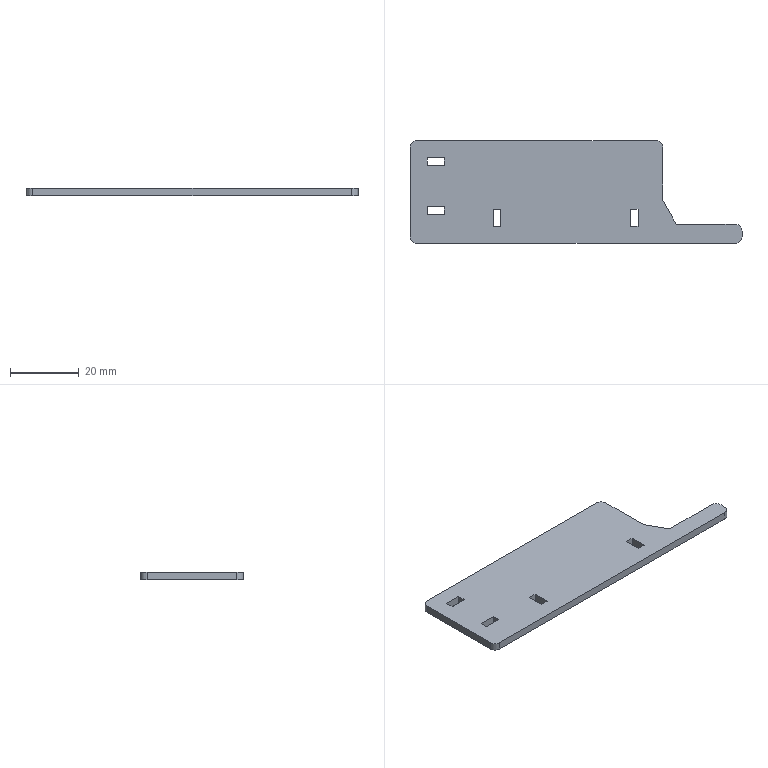Part | SolidWorks | features FlatPattern 1, SMBaseFlange 1, SheetMetal 1 | 1 solid | 31 faces | box 96.8 x 30.001 x 2.3 mm | volume 5301 mm3 | plane 25 | cylinder 6 | commonest cylinder face diameters 4 x6
STEP:
#1=CARTESIAN_POINT('',(1194.712,-717.303,2.3));
#2=VERTEX_POINT('',#1);
#3=CARTESIAN_POINT('',(1196.712,-719.303,2.3));
#4=VERTEX_POINT('',#3);
#5=CARTESIAN_POINT('',(1196.712,-717.303,2.3));
#6=DIRECTION('',(0.,0.,1.));
#7=DIRECTION('',(1.,0.,0.));
#8=AXIS2_PLACEMENT_3D('',#5,#6,#7);
#9=CIRCLE('',#8,2.);
#10=EDGE_CURVE('',#2,#4,#9,.T.);
#11=ORIENTED_EDGE('',*,*,#10,.F.);
#12=CARTESIAN_POINT('',(1194.712,-717.303,0.));
#13=VERTEX_POINT('',#12);
#14=CARTESIAN_POINT('',(1194.712,-717.303,2.3));
#15=DIRECTION('',(0.,0.,-1.));
#16=VECTOR('',#15,1000.);
#17=LINE('',#14,#16);
#18=EDGE_CURVE('',#2,#13,#17,.T.);
#19=ORIENTED_EDGE('',*,*,#18,.T.);
#20=CARTESIAN_POINT('',(1196.712,-719.303,0.));
#21=VERTEX_POINT('',#20);
#22=CARTESIAN_POINT('',(1196.712,-717.303,0.));
#23=DIRECTION('',(0.,0.,1.));
#24=DIRECTION('',(1.,0.,0.));
#25=AXIS2_PLACEMENT_3D('',#22,#23,#24);
#26=CIRCLE('',#25,2.);
#27=EDGE_CURVE('',#13,#21,#26,.T.);
#28=ORIENTED_EDGE('',*,*,#27,.T.);
#29=CARTESIAN_POINT('',(1196.712,-719.303,2.3));
#30=DIRECTION('',(0.,0.,-1.));
#31=VECTOR('',#30,1000.);
#32=LINE('',#29,#31);
#33=EDGE_CURVE('',#4,#21,#32,.T.);
#34=ORIENTED_EDGE('',*,*,#33,.F.);
#35=EDGE_LOOP('',(#11,#19,#28,#34));
#36=FACE_OUTER_BOUND('',#35,.T.);
#37=CARTESIAN_POINT('',(1196.712,-717.303,2.3));
#38=DIRECTION('',(0.,0.,-1.));
#39=DIRECTION('',(-1.,0.,0.));
#40=AXIS2_PLACEMENT_3D('',#37,#38,#39);
#41=CYLINDRICAL_SURFACE('',#40,2.);
#42=ADVANCED_FACE('',(#36),#41,.T.);
#43=CARTESIAN_POINT('',(1272.362,-713.702,2.3));
#44=VERTEX_POINT('',#43);
#45=CARTESIAN_POINT('',(1268.452,-706.712,2.3));
#46=VERTEX_POINT('',#45);
#47=CARTESIAN_POINT('',(1272.362,-713.702,2.3));
#48=DIRECTION('',(-0.4882,0.8727,0.));
#49=VECTOR('',#48,1000.);
#50=LINE('',#47,#49);
#51=EDGE_CURVE('',#44,#46,#50,.T.);
#52=ORIENTED_EDGE('',*,*,#51,.T.);
#53=CARTESIAN_POINT('',(1268.452,-691.303,2.3));
#54=VERTEX_POINT('',#53);
#55=CARTESIAN_POINT('',(1268.452,-706.712,2.3));
#56=DIRECTION('',(0.,1.,0.));
#57=VECTOR('',#56,1000.);
#58=LINE('',#55,#57);
#59=EDGE_CURVE('',#46,#54,#58,.T.);
#60=ORIENTED_EDGE('',*,*,#59,.T.);
#61=CARTESIAN_POINT('',(1266.452,-689.303,2.3));
#62=VERTEX_POINT('',#61);
#63=CARTESIAN_POINT('',(1266.452,-691.303,2.3));
#64=DIRECTION('',(0.,0.,1.));
#65=DIRECTION('',(1.,0.,0.));
#66=AXIS2_PLACEMENT_3D('',#63,#64,#65);
#67=CIRCLE('',#66,2.);
#68=EDGE_CURVE('',#54,#62,#67,.T.);
#69=ORIENTED_EDGE('',*,*,#68,.T.);
#70=CARTESIAN_POINT('',(1196.712,-689.303,2.3));
#71=VERTEX_POINT('',#70);
#72=CARTESIAN_POINT('',(1266.452,-689.303,2.3));
#73=DIRECTION('',(-1.,0.,0.));
#74=VECTOR('',#73,1000.);
#75=LINE('',#72,#74);
#76=EDGE_CURVE('',#62,#71,#75,.T.);
#77=ORIENTED_EDGE('',*,*,#76,.T.);
#78=CARTESIAN_POINT('',(1194.712,-691.303,2.3));
#79=VERTEX_POINT('',#78);
#80=CARTESIAN_POINT('',(1196.712,-691.303,2.3));
#81=DIRECTION('',(0.,0.,1.));
#82=DIRECTION('',(1.,0.,0.));
#83=AXIS2_PLACEMENT_3D('',#80,#81,#82);
#84=CIRCLE('',#83,2.);
#85=EDGE_CURVE('',#71,#79,#84,.T.);
#86=ORIENTED_EDGE('',*,*,#85,.T.);
#87=CARTESIAN_POINT('',(1194.712,-717.303,2.3));
#88=VERTEX_POINT('',#87);
#89=CARTESIAN_POINT('',(1194.712,-691.303,2.3));
#90=DIRECTION('',(-0.00001077,-1.,0.));
#91=VECTOR('',#90,1000.);
#92=LINE('',#89,#91);
#93=EDGE_CURVE('',#79,#88,#92,.T.);
#94=ORIENTED_EDGE('',*,*,#93,.T.);
#95=CARTESIAN_POINT('',(1196.712,-717.303,2.3));
#96=DIRECTION('',(0.,0.,1.));
#97=DIRECTION('',(1.,0.,0.));
#98=AXIS2_PLACEMENT_3D('',#95,#96,#97);
#99=CIRCLE('',#98,2.);
#100=EDGE_CURVE('',#88,#2,#99,.T.);
#101=ORIENTED_EDGE('',*,*,#100,.T.);
#102=ORIENTED_EDGE('',*,*,#10,.T.);
#103=CARTESIAN_POINT('',(1289.512,-719.303,2.3));
#104=VERTEX_POINT('',#103);
#105=CARTESIAN_POINT('',(1196.712,-719.303,2.3));
#106=DIRECTION('',(1.,-0.000005963,0.));
#107=VECTOR('',#106,1000.);
#108=LINE('',#105,#107);
#109=EDGE_CURVE('',#4,#104,#108,.T.);
#110=ORIENTED_EDGE('',*,*,#109,.T.);
#111=CARTESIAN_POINT('',(1291.512,-717.303,2.3));
#112=VERTEX_POINT('',#111);
#113=CARTESIAN_POINT('',(1289.512,-717.303,2.3));
#114=DIRECTION('',(0.,0.,1.));
#115=DIRECTION('',(-1.,0.,0.));
#116=AXIS2_PLACEMENT_3D('',#113,#114,#115);
#117=CIRCLE('',#116,2.);
#118=EDGE_CURVE('',#104,#112,#117,.T.);
#119=ORIENTED_EDGE('',*,*,#118,.T.);
#120=CARTESIAN_POINT('',(1291.512,-715.702,2.3));
#121=VERTEX_POINT('',#120);
#122=CARTESIAN_POINT('',(1291.512,-715.702,2.3));
#123=DIRECTION('',(0.,1.,0.));
#124=VECTOR('',#123,1000.);
#125=LINE('',#122,#124);
#126=EDGE_CURVE('',#112,#121,#125,.T.);
#127=ORIENTED_EDGE('',*,*,#126,.T.);
#128=CARTESIAN_POINT('',(1289.512,-713.702,2.3));
#129=VERTEX_POINT('',#128);
#130=CARTESIAN_POINT('',(1289.512,-715.702,2.3));
#131=DIRECTION('',(0.,0.,1.));
#132=DIRECTION('',(1.,0.,0.));
#133=AXIS2_PLACEMENT_3D('',#130,#131,#132);
#134=CIRCLE('',#133,2.);
#135=EDGE_CURVE('',#121,#129,#134,.T.);
#136=ORIENTED_EDGE('',*,*,#135,.T.);
#137=CARTESIAN_POINT('',(1289.512,-713.702,2.3));
#138=DIRECTION('',(-1.,0.,0.));
#139=VECTOR('',#138,1000.);
#140=LINE('',#137,#139);
#141=EDGE_CURVE('',#129,#44,#140,.T.);
#142=ORIENTED_EDGE('',*,*,#141,.T.);
#143=EDGE_LOOP('',(#52,#60,#69,#77,#86,#94,#101,#102,#110,#119,#127,#136,#142));
#144=FACE_OUTER_BOUND('',#143,.T.);
#145=CARTESIAN_POINT('',(1218.912,-714.303,2.3));
#146=VERTEX_POINT('',#145);
#147=CARTESIAN_POINT('',(1221.212,-714.303,2.3));
#148=VERTEX_POINT('',#147);
#149=CARTESIAN_POINT('',(1218.912,-714.303,2.3));
#150=DIRECTION('',(1.,0.,0.));
#151=VECTOR('',#150,1000.);
#152=LINE('',#149,#151);
#153=EDGE_CURVE('',#146,#148,#152,.T.);
#154=ORIENTED_EDGE('',*,*,#153,.F.);
#155=CARTESIAN_POINT('',(1218.912,-709.303,2.3));
#156=VERTEX_POINT('',#155);
#157=CARTESIAN_POINT('',(1218.912,-709.303,2.3));
#158=DIRECTION('',(0.,-1.,0.));
#159=VECTOR('',#158,1000.);
#160=LINE('',#157,#159);
#161=EDGE_CURVE('',#156,#146,#160,.T.);
#162=ORIENTED_EDGE('',*,*,#161,.F.);
#163=CARTESIAN_POINT('',(1221.212,-709.303,2.3));
#164=VERTEX_POINT('',#163);
#165=CARTESIAN_POINT('',(1218.912,-709.303,2.3));
#166=DIRECTION('',(-1.,0.,0.));
#167=VECTOR('',#166,1000.);
#168=LINE('',#165,#167);
#169=EDGE_CURVE('',#164,#156,#168,.T.);
#170=ORIENTED_EDGE('',*,*,#169,.F.);
#171=CARTESIAN_POINT('',(1221.212,-709.303,2.3));
#172=DIRECTION('',(0.,1.,0.));
#173=VECTOR('',#172,1000.);
#174=LINE('',#171,#173);
#175=EDGE_CURVE('',#148,#164,#174,.T.);
#176=ORIENTED_EDGE('',*,*,#175,.F.);
#177=EDGE_LOOP('',(#154,#162,#170,#176));
#178=FACE_BOUND('',#177,.T.);
#179=CARTESIAN_POINT('',(1258.912,-714.303,2.3));
#180=VERTEX_POINT('',#179);
#181=CARTESIAN_POINT('',(1261.212,-714.303,2.3));
#182=VERTEX_POINT('',#181);
#183=CARTESIAN_POINT('',(1258.912,-714.303,2.3));
#184=DIRECTION('',(1.,0.,0.));
#185=VECTOR('',#184,1000.);
#186=LINE('',#183,#185);
#187=EDGE_CURVE('',#180,#182,#186,.T.);
#188=ORIENTED_EDGE('',*,*,#187,.F.);
#189=CARTESIAN_POINT('',(1258.912,-709.303,2.3));
#190=VERTEX_POINT('',#189);
#191=CARTESIAN_POINT('',(1258.912,-709.303,2.3));
#192=DIRECTION('',(0.,-1.,0.));
#193=VECTOR('',#192,1000.);
#194=LINE('',#191,#193);
#195=EDGE_CURVE('',#190,#180,#194,.T.);
#196=ORIENTED_EDGE('',*,*,#195,.F.);
#197=CARTESIAN_POINT('',(1261.212,-709.303,2.3));
#198=VERTEX_POINT('',#197);
#199=CARTESIAN_POINT('',(1258.912,-709.303,2.3));
#200=DIRECTION('',(-1.,0.,0.));
#201=VECTOR('',#200,1000.);
#202=LINE('',#199,#201);
#203=EDGE_CURVE('',#198,#190,#202,.T.);
#204=ORIENTED_EDGE('',*,*,#203,.F.);
#205=CARTESIAN_POINT('',(1261.212,-709.303,2.3));
#206=DIRECTION('',(0.,1.,0.));
#207=VECTOR('',#206,1000.);
#208=LINE('',#205,#207);
#209=EDGE_CURVE('',#182,#198,#208,.T.);
#210=ORIENTED_EDGE('',*,*,#209,.F.);
#211=EDGE_LOOP('',(#188,#196,#204,#210));
#212=FACE_BOUND('',#211,.T.);
#213=CARTESIAN_POINT('',(1199.712,-696.603,2.3));
#214=VERTEX_POINT('',#213);
#215=CARTESIAN_POINT('',(1204.712,-696.603,2.3));
#216=VERTEX_POINT('',#215);
#217=CARTESIAN_POINT('',(1199.712,-696.603,2.3));
#218=DIRECTION('',(1.,0.,0.));
#219=VECTOR('',#218,1000.);
#220=LINE('',#217,#219);
#221=EDGE_CURVE('',#214,#216,#220,.T.);
#222=ORIENTED_EDGE('',*,*,#221,.F.);
#223=CARTESIAN_POINT('',(1199.712,-694.303,2.3));
#224=VERTEX_POINT('',#223);
#225=CARTESIAN_POINT('',(1199.712,-694.303,2.3));
#226=DIRECTION('',(0.,-1.,0.));
#227=VECTOR('',#226,1000.);
#228=LINE('',#225,#227);
#229=EDGE_CURVE('',#224,#214,#228,.T.);
#230=ORIENTED_EDGE('',*,*,#229,.F.);
#231=CARTESIAN_POINT('',(1204.712,-694.303,2.3));
#232=VERTEX_POINT('',#231);
#233=CARTESIAN_POINT('',(1199.712,-694.303,2.3));
#234=DIRECTION('',(-1.,0.,0.));
#235=VECTOR('',#234,1000.);
#236=LINE('',#233,#235);
#237=EDGE_CURVE('',#232,#224,#236,.T.);
#238=ORIENTED_EDGE('',*,*,#237,.F.);
#239=CARTESIAN_POINT('',(1204.712,-694.303,2.3));
#240=DIRECTION('',(0.,1.,0.));
#241=VECTOR('',#240,1000.);
#242=LINE('',#239,#241);
#243=EDGE_CURVE('',#216,#232,#242,.T.);
#244=ORIENTED_EDGE('',*,*,#243,.F.);
#245=EDGE_LOOP('',(#222,#230,#238,#244));
#246=FACE_BOUND('',#245,.T.);
#247=CARTESIAN_POINT('',(1199.712,-710.903,2.3));
#248=VERTEX_POINT('',#247);
#249=CARTESIAN_POINT('',(1204.712,-710.903,2.3));
#250=VERTEX_POINT('',#249);
#251=CARTESIAN_POINT('',(1199.712,-710.903,2.3));
#252=DIRECTION('',(1.,0.,0.));
#253=VECTOR('',#252,1000.);
#254=LINE('',#251,#253);
#255=EDGE_CURVE('',#248,#250,#254,.T.);
#256=ORIENTED_EDGE('',*,*,#255,.F.);
#257=CARTESIAN_POINT('',(1199.712,-708.603,2.3));
#258=VERTEX_POINT('',#257);
#259=CARTESIAN_POINT('',(1199.712,-708.603,2.3));
#260=DIRECTION('',(0.,-1.,0.));
#261=VECTOR('',#260,1000.);
#262=LINE('',#259,#261);
#263=EDGE_CURVE('',#258,#248,#262,.T.);
#264=ORIENTED_EDGE('',*,*,#263,.F.);
#265=CARTESIAN_POINT('',(1204.712,-708.603,2.3));
#266=VERTEX_POINT('',#265);
#267=CARTESIAN_POINT('',(1199.712,-708.603,2.3));
#268=DIRECTION('',(-1.,0.,0.));
#269=VECTOR('',#268,1000.);
#270=LINE('',#267,#269);
#271=EDGE_CURVE('',#266,#258,#270,.T.);
#272=ORIENTED_EDGE('',*,*,#271,.F.);
#273=CARTESIAN_POINT('',(1204.712,-708.603,2.3));
#274=DIRECTION('',(0.,1.,0.));
#275=VECTOR('',#274,1000.);
#276=LINE('',#273,#275);
#277=EDGE_CURVE('',#250,#266,#276,.T.);
#278=ORIENTED_EDGE('',*,*,#277,.F.);
#279=EDGE_LOOP('',(#256,#264,#272,#278));
#280=FACE_BOUND('',#279,.T.);
#281=CARTESIAN_POINT('',(1266.452,-691.303,2.3));
#282=DIRECTION('',(0.,0.,1.));
#283=DIRECTION('',(1.,0.,0.));
#284=AXIS2_PLACEMENT_3D('',#281,#282,#283);
#285=PLANE('',#284);
#286=ADVANCED_FACE('',(#144,#178,#212,#246,#280),#285,.T.);
#287=CARTESIAN_POINT('',(1199.712,-694.303,0.));
#288=VERTEX_POINT('',#287);
#289=CARTESIAN_POINT('',(1199.712,-696.603,0.));
#290=VERTEX_POINT('',#289);
#291=CARTESIAN_POINT('',(1199.712,-694.303,0.));
#292=DIRECTION('',(0.,-1.,0.));
#293=VECTOR('',#292,1000.);
#294=LINE('',#291,#293);
#295=EDGE_CURVE('',#288,#290,#294,.T.);
#296=ORIENTED_EDGE('',*,*,#295,.T.);
#297=CARTESIAN_POINT('',(1204.712,-696.603,0.));
#298=VERTEX_POINT('',#297);
#299=CARTESIAN_POINT('',(1199.712,-696.603,0.));
#300=DIRECTION('',(1.,0.,0.));
#301=VECTOR('',#300,1000.);
#302=LINE('',#299,#301);
#303=EDGE_CURVE('',#290,#298,#302,.T.);
#304=ORIENTED_EDGE('',*,*,#303,.T.);
#305=CARTESIAN_POINT('',(1204.712,-694.303,0.));
#306=VERTEX_POINT('',#305);
#307=CARTESIAN_POINT('',(1204.712,-694.303,0.));
#308=DIRECTION('',(0.,1.,0.));
#309=VECTOR('',#308,1000.);
#310=LINE('',#307,#309);
#311=EDGE_CURVE('',#298,#306,#310,.T.);
#312=ORIENTED_EDGE('',*,*,#311,.T.);
#313=CARTESIAN_POINT('',(1199.712,-694.303,0.));
#314=DIRECTION('',(-1.,0.,0.));
#315=VECTOR('',#314,1000.);
#316=LINE('',#313,#315);
#317=EDGE_CURVE('',#306,#288,#316,.T.);
#318=ORIENTED_EDGE('',*,*,#317,.T.);
#319=EDGE_LOOP('',(#296,#304,#312,#318));
#320=FACE_BOUND('',#319,.T.);
#321=CARTESIAN_POINT('',(1218.912,-709.303,0.));
#322=VERTEX_POINT('',#321);
#323=CARTESIAN_POINT('',(1218.912,-714.303,0.));
#324=VERTEX_POINT('',#323);
#325=CARTESIAN_POINT('',(1218.912,-709.303,0.));
#326=DIRECTION('',(0.,-1.,0.));
#327=VECTOR('',#326,1000.);
#328=LINE('',#325,#327);
#329=EDGE_CURVE('',#322,#324,#328,.T.);
#330=ORIENTED_EDGE('',*,*,#329,.T.);
#331=CARTESIAN_POINT('',(1221.212,-714.303,0.));
#332=VERTEX_POINT('',#331);
#333=CARTESIAN_POINT('',(1218.912,-714.303,0.));
#334=DIRECTION('',(1.,0.,0.));
#335=VECTOR('',#334,1000.);
#336=LINE('',#333,#335);
#337=EDGE_CURVE('',#324,#332,#336,.T.);
#338=ORIENTED_EDGE('',*,*,#337,.T.);
#339=CARTESIAN_POINT('',(1221.212,-709.303,0.));
#340=VERTEX_POINT('',#339);
#341=CARTESIAN_POINT('',(1221.212,-709.303,0.));
#342=DIRECTION('',(0.,1.,0.));
#343=VECTOR('',#342,1000.);
#344=LINE('',#341,#343);
#345=EDGE_CURVE('',#332,#340,#344,.T.);
#346=ORIENTED_EDGE('',*,*,#345,.T.);
#347=CARTESIAN_POINT('',(1218.912,-709.303,0.));
#348=DIRECTION('',(-1.,0.,0.));
#349=VECTOR('',#348,1000.);
#350=LINE('',#347,#349);
#351=EDGE_CURVE('',#340,#322,#350,.T.);
#352=ORIENTED_EDGE('',*,*,#351,.T.);
#353=EDGE_LOOP('',(#330,#338,#346,#352));
#354=FACE_BOUND('',#353,.T.);
#355=CARTESIAN_POINT('',(1272.362,-713.702,0.));
#356=VERTEX_POINT('',#355);
#357=CARTESIAN_POINT('',(1268.452,-706.712,0.));
#358=VERTEX_POINT('',#357);
#359=CARTESIAN_POINT('',(1272.362,-713.702,0.));
#360=DIRECTION('',(-0.4882,0.8727,0.));
#361=VECTOR('',#360,1000.);
#362=LINE('',#359,#361);
#363=EDGE_CURVE('',#356,#358,#362,.T.);
#364=ORIENTED_EDGE('',*,*,#363,.F.);
#365=CARTESIAN_POINT('',(1289.512,-713.702,0.));
#366=VERTEX_POINT('',#365);
#367=CARTESIAN_POINT('',(1289.512,-713.702,0.));
#368=DIRECTION('',(-1.,0.,0.));
#369=VECTOR('',#368,1000.);
#370=LINE('',#367,#369);
#371=EDGE_CURVE('',#366,#356,#370,.T.);
#372=ORIENTED_EDGE('',*,*,#371,.F.);
#373=CARTESIAN_POINT('',(1291.512,-715.702,0.));
#374=VERTEX_POINT('',#373);
#375=CARTESIAN_POINT('',(1289.512,-715.702,0.));
#376=DIRECTION('',(0.,0.,1.));
#377=DIRECTION('',(1.,0.,0.));
#378=AXIS2_PLACEMENT_3D('',#375,#376,#377);
#379=CIRCLE('',#378,2.);
#380=EDGE_CURVE('',#374,#366,#379,.T.);
#381=ORIENTED_EDGE('',*,*,#380,.F.);
#382=CARTESIAN_POINT('',(1291.512,-717.303,0.));
#383=VERTEX_POINT('',#382);
#384=CARTESIAN_POINT('',(1291.512,-715.702,0.));
#385=DIRECTION('',(0.,1.,0.));
#386=VECTOR('',#385,1000.);
#387=LINE('',#384,#386);
#388=EDGE_CURVE('',#383,#374,#387,.T.);
#389=ORIENTED_EDGE('',*,*,#388,.F.);
#390=CARTESIAN_POINT('',(1289.512,-719.303,0.));
#391=VERTEX_POINT('',#390);
#392=CARTESIAN_POINT('',(1289.512,-717.303,0.));
#393=DIRECTION('',(0.,0.,1.));
#394=DIRECTION('',(-1.,0.,0.));
#395=AXIS2_PLACEMENT_3D('',#392,#393,#394);
#396=CIRCLE('',#395,2.);
#397=EDGE_CURVE('',#391,#383,#396,.T.);
#398=ORIENTED_EDGE('',*,*,#397,.F.);
#399=CARTESIAN_POINT('',(1196.712,-719.303,0.));
#400=DIRECTION('',(1.,-0.000005963,0.));
#401=VECTOR('',#400,1000.);
#402=LINE('',#399,#401);
#403=EDGE_CURVE('',#21,#391,#402,.T.);
#404=ORIENTED_EDGE('',*,*,#403,.F.);
#405=ORIENTED_EDGE('',*,*,#27,.F.);
#406=CARTESIAN_POINT('',(1194.712,-717.303,0.));
#407=VERTEX_POINT('',#406);
#408=CARTESIAN_POINT('',(1196.712,-717.303,0.));
#409=DIRECTION('',(0.,0.,1.));
#410=DIRECTION('',(1.,0.,0.));
#411=AXIS2_PLACEMENT_3D('',#408,#409,#410);
#412=CIRCLE('',#411,2.);
#413=EDGE_CURVE('',#407,#13,#412,.T.);
#414=ORIENTED_EDGE('',*,*,#413,.F.);
#415=CARTESIAN_POINT('',(1194.712,-691.303,0.));
#416=VERTEX_POINT('',#415);
#417=CARTESIAN_POINT('',(1194.712,-691.303,0.));
#418=DIRECTION('',(-0.00001077,-1.,0.));
#419=VECTOR('',#418,1000.);
#420=LINE('',#417,#419);
#421=EDGE_CURVE('',#416,#407,#420,.T.);
#422=ORIENTED_EDGE('',*,*,#421,.F.);
#423=CARTESIAN_POINT('',(1196.712,-689.303,0.));
#424=VERTEX_POINT('',#423);
#425=CARTESIAN_POINT('',(1196.712,-691.303,0.));
#426=DIRECTION('',(0.,0.,1.));
#427=DIRECTION('',(1.,0.,0.));
#428=AXIS2_PLACEMENT_3D('',#425,#426,#427);
#429=CIRCLE('',#428,2.);
#430=EDGE_CURVE('',#424,#416,#429,.T.);
#431=ORIENTED_EDGE('',*,*,#430,.F.);
#432=CARTESIAN_POINT('',(1266.452,-689.303,0.));
#433=VERTEX_POINT('',#432);
#434=CARTESIAN_POINT('',(1266.452,-689.303,0.));
#435=DIRECTION('',(-1.,0.,0.));
#436=VECTOR('',#435,1000.);
#437=LINE('',#434,#436);
#438=EDGE_CURVE('',#433,#424,#437,.T.);
#439=ORIENTED_EDGE('',*,*,#438,.F.);
#440=CARTESIAN_POINT('',(1268.452,-691.303,0.));
#441=VERTEX_POINT('',#440);
#442=CARTESIAN_POINT('',(1266.452,-691.303,0.));
#443=DIRECTION('',(0.,0.,1.));
#444=DIRECTION('',(1.,0.,0.));
#445=AXIS2_PLACEMENT_3D('',#442,#443,#444);
#446=CIRCLE('',#445,2.);
#447=EDGE_CURVE('',#441,#433,#446,.T.);
#448=ORIENTED_EDGE('',*,*,#447,.F.);
#449=CARTESIAN_POINT('',(1268.452,-706.712,0.));
#450=DIRECTION('',(0.,1.,0.));
#451=VECTOR('',#450,1000.);
#452=LINE('',#449,#451);
#453=EDGE_CURVE('',#358,#441,#452,.T.);
#454=ORIENTED_EDGE('',*,*,#453,.F.);
#455=EDGE_LOOP('',(#364,#372,#381,#389,#398,#404,#405,#414,#422,#431,#439,#448,#454));
#456=FACE_OUTER_BOUND('',#455,.T.);
#457=CARTESIAN_POINT('',(1258.912,-709.303,0.));
#458=VERTEX_POINT('',#457);
#459=CARTESIAN_POINT('',(1258.912,-714.303,0.));
#460=VERTEX_POINT('',#459);
#461=CARTESIAN_POINT('',(1258.912,-709.303,0.));
#462=DIRECTION('',(0.,-1.,0.));
#463=VECTOR('',#462,1000.);
#464=LINE('',#461,#463);
#465=EDGE_CURVE('',#458,#460,#464,.T.);
#466=ORIENTED_EDGE('',*,*,#465,.T.);
#467=CARTESIAN_POINT('',(1261.212,-714.303,0.));
#468=VERTEX_POINT('',#467);
#469=CARTESIAN_POINT('',(1258.912,-714.303,0.));
#470=DIRECTION('',(1.,0.,0.));
#471=VECTOR('',#470,1000.);
#472=LINE('',#469,#471);
#473=EDGE_CURVE('',#460,#468,#472,.T.);
#474=ORIENTED_EDGE('',*,*,#473,.T.);
#475=CARTESIAN_POINT('',(1261.212,-709.303,0.));
#476=VERTEX_POINT('',#475);
#477=CARTESIAN_POINT('',(1261.212,-709.303,0.));
#478=DIRECTION('',(0.,1.,0.));
#479=VECTOR('',#478,1000.);
#480=LINE('',#477,#479);
#481=EDGE_CURVE('',#468,#476,#480,.T.);
#482=ORIENTED_EDGE('',*,*,#481,.T.);
#483=CARTESIAN_POINT('',(1258.912,-709.303,0.));
#484=DIRECTION('',(-1.,0.,0.));
#485=VECTOR('',#484,1000.);
#486=LINE('',#483,#485);
#487=EDGE_CURVE('',#476,#458,#486,.T.);
#488=ORIENTED_EDGE('',*,*,#487,.T.);
#489=EDGE_LOOP('',(#466,#474,#482,#488));
#490=FACE_BOUND('',#489,.T.);
#491=CARTESIAN_POINT('',(1199.712,-708.603,0.));
#492=VERTEX_POINT('',#491);
#493=CARTESIAN_POINT('',(1199.712,-710.903,0.));
#494=VERTEX_POINT('',#493);
#495=CARTESIAN_POINT('',(1199.712,-708.603,0.));
#496=DIRECTION('',(0.,-1.,0.));
#497=VECTOR('',#496,1000.);
#498=LINE('',#495,#497);
#499=EDGE_CURVE('',#492,#494,#498,.T.);
#500=ORIENTED_EDGE('',*,*,#499,.T.);
#501=CARTESIAN_POINT('',(1204.712,-710.903,0.));
#502=VERTEX_POINT('',#501);
#503=CARTESIAN_POINT('',(1199.712,-710.903,0.));
#504=DIRECTION('',(1.,0.,0.));
#505=VECTOR('',#504,1000.);
#506=LINE('',#503,#505);
#507=EDGE_CURVE('',#494,#502,#506,.T.);
#508=ORIENTED_EDGE('',*,*,#507,.T.);
#509=CARTESIAN_POINT('',(1204.712,-708.603,0.));
#510=VERTEX_POINT('',#509);
#511=CARTESIAN_POINT('',(1204.712,-708.603,0.));
#512=DIRECTION('',(0.,1.,0.));
#513=VECTOR('',#512,1000.);
#514=LINE('',#511,#513);
#515=EDGE_CURVE('',#502,#510,#514,.T.);
#516=ORIENTED_EDGE('',*,*,#515,.T.);
#517=CARTESIAN_POINT('',(1199.712,-708.603,0.));
#518=DIRECTION('',(-1.,0.,0.));
#519=VECTOR('',#518,1000.);
#520=LINE('',#517,#519);
#521=EDGE_CURVE('',#510,#492,#520,.T.);
#522=ORIENTED_EDGE('',*,*,#521,.T.);
#523=EDGE_LOOP('',(#500,#508,#516,#522));
#524=FACE_BOUND('',#523,.T.);
#525=CARTESIAN_POINT('',(1266.452,-691.303,0.));
#526=DIRECTION('',(0.,0.,1.));
#527=DIRECTION('',(1.,0.,0.));
#528=AXIS2_PLACEMENT_3D('',#525,#526,#527);
#529=PLANE('',#528);
#530=ADVANCED_FACE('',(#320,#354,#456,#490,#524),#529,.F.);
#531=ORIENTED_EDGE('',*,*,#363,.T.);
#532=CARTESIAN_POINT('',(1268.452,-706.712,2.3));
#533=DIRECTION('',(0.,0.,-1.));
#534=VECTOR('',#533,1000.);
#535=LINE('',#532,#534);
#536=EDGE_CURVE('',#46,#358,#535,.T.);
#537=ORIENTED_EDGE('',*,*,#536,.F.);
#538=ORIENTED_EDGE('',*,*,#51,.F.);
#539=CARTESIAN_POINT('',(1272.362,-713.702,2.3));
#540=DIRECTION('',(0.,0.,-1.));
#541=VECTOR('',#540,1000.);
#542=LINE('',#539,#541);
#543=EDGE_CURVE('',#44,#356,#542,.T.);
#544=ORIENTED_EDGE('',*,*,#543,.T.);
#545=EDGE_LOOP('',(#531,#537,#538,#544));
#546=FACE_OUTER_BOUND('',#545,.T.);
#547=CARTESIAN_POINT('',(1272.362,-713.702,2.3));
#548=DIRECTION('',(-0.8727,-0.4882,0.));
#549=DIRECTION('',(0.4882,-0.8727,0.));
#550=AXIS2_PLACEMENT_3D('',#547,#548,#549);
#551=PLANE('',#550);
#552=ADVANCED_FACE('',(#546),#551,.F.);
#553=ORIENTED_EDGE('',*,*,#453,.T.);
#554=CARTESIAN_POINT('',(1268.452,-691.303,2.3));
#555=DIRECTION('',(0.,0.,-1.));
#556=VECTOR('',#555,1000.);
#557=LINE('',#554,#556);
#558=EDGE_CURVE('',#54,#441,#557,.T.);
#559=ORIENTED_EDGE('',*,*,#558,.F.);
#560=ORIENTED_EDGE('',*,*,#59,.F.);
#561=ORIENTED_EDGE('',*,*,#536,.T.);
#562=EDGE_LOOP('',(#553,#559,#560,#561));
#563=FACE_OUTER_BOUND('',#562,.T.);
#564=CARTESIAN_POINT('',(1268.452,-706.712,2.3));
#565=DIRECTION('',(-1.,0.,0.));
#566=DIRECTION('',(0.,-1.,0.));
#567=AXIS2_PLACEMENT_3D('',#564,#565,#566);
#568=PLANE('',#567);
#569=ADVANCED_FACE('',(#563),#568,.F.);
#570=ORIENTED_EDGE('',*,*,#447,.T.);
#571=CARTESIAN_POINT('',(1266.452,-689.303,2.3));
#572=DIRECTION('',(0.,0.,-1.));
#573=VECTOR('',#572,1000.);
#574=LINE('',#571,#573);
#575=EDGE_CURVE('',#62,#433,#574,.T.);
#576=ORIENTED_EDGE('',*,*,#575,.F.);
#577=ORIENTED_EDGE('',*,*,#68,.F.);
#578=ORIENTED_EDGE('',*,*,#558,.T.);
#579=EDGE_LOOP('',(#570,#576,#577,#578));
#580=FACE_OUTER_BOUND('',#579,.T.);
#581=CARTESIAN_POINT('',(1266.452,-691.303,2.3));
#582=DIRECTION('',(0.,0.,-1.));
#583=DIRECTION('',(-1.,0.,0.));
#584=AXIS2_PLACEMENT_3D('',#581,#582,#583);
#585=CYLINDRICAL_SURFACE('',#584,2.);
#586=ADVANCED_FACE('',(#580),#585,.T.);
#587=ORIENTED_EDGE('',*,*,#438,.T.);
#588=CARTESIAN_POINT('',(1196.712,-689.303,2.3));
#589=DIRECTION('',(0.,0.,-1.));
#590=VECTOR('',#589,1000.);
#591=LINE('',#588,#590);
#592=EDGE_CURVE('',#71,#424,#591,.T.);
#593=ORIENTED_EDGE('',*,*,#592,.F.);
#594=ORIENTED_EDGE('',*,*,#76,.F.);
#595=ORIENTED_EDGE('',*,*,#575,.T.);
#596=EDGE_LOOP('',(#587,#593,#594,#595));
#597=FACE_OUTER_BOUND('',#596,.T.);
#598=CARTESIAN_POINT('',(1266.452,-689.303,2.3));
#599=DIRECTION('',(0.,-1.,0.));
#600=DIRECTION('',(1.,0.,0.));
#601=AXIS2_PLACEMENT_3D('',#598,#599,#600);
#602=PLANE('',#601);
#603=ADVANCED_FACE('',(#597),#602,.F.);
#604=ORIENTED_EDGE('',*,*,#430,.T.);
#605=CARTESIAN_POINT('',(1194.712,-691.303,2.3));
#606=DIRECTION('',(0.,0.,-1.));
#607=VECTOR('',#606,1000.);
#608=LINE('',#605,#607);
#609=EDGE_CURVE('',#79,#416,#608,.T.);
#610=ORIENTED_EDGE('',*,*,#609,.F.);
#611=ORIENTED_EDGE('',*,*,#85,.F.);
#612=ORIENTED_EDGE('',*,*,#592,.T.);
#613=EDGE_LOOP('',(#604,#610,#611,#612));
#614=FACE_OUTER_BOUND('',#613,.T.);
#615=CARTESIAN_POINT('',(1196.712,-691.303,2.3));
#616=DIRECTION('',(0.,0.,-1.));
#617=DIRECTION('',(-1.,0.,0.));
#618=AXIS2_PLACEMENT_3D('',#615,#616,#617);
#619=CYLINDRICAL_SURFACE('',#618,2.);
#620=ADVANCED_FACE('',(#614),#619,.T.);
#621=ORIENTED_EDGE('',*,*,#421,.T.);
#622=CARTESIAN_POINT('',(1194.712,-717.303,2.3));
#623=DIRECTION('',(0.,0.,-1.));
#624=VECTOR('',#623,1000.);
#625=LINE('',#622,#624);
#626=EDGE_CURVE('',#88,#407,#625,.T.);
#627=ORIENTED_EDGE('',*,*,#626,.F.);
#628=ORIENTED_EDGE('',*,*,#93,.F.);
#629=ORIENTED_EDGE('',*,*,#609,.T.);
#630=EDGE_LOOP('',(#621,#627,#628,#629));
#631=FACE_OUTER_BOUND('',#630,.T.);
#632=CARTESIAN_POINT('',(1194.712,-691.303,2.3));
#633=DIRECTION('',(1.,-0.00001077,0.));
#634=DIRECTION('',(0.00001077,1.,0.));
#635=AXIS2_PLACEMENT_3D('',#632,#633,#634);
#636=PLANE('',#635);
#637=ADVANCED_FACE('',(#631),#636,.F.);
#638=ORIENTED_EDGE('',*,*,#18,.F.);
#639=ORIENTED_EDGE('',*,*,#100,.F.);
#640=ORIENTED_EDGE('',*,*,#626,.T.);
#641=ORIENTED_EDGE('',*,*,#413,.T.);
#642=EDGE_LOOP('',(#638,#639,#640,#641));
#643=FACE_OUTER_BOUND('',#642,.T.);
#644=CARTESIAN_POINT('',(1196.712,-717.303,2.3));
#645=DIRECTION('',(0.,0.,-1.));
#646=DIRECTION('',(-1.,0.,0.));
#647=AXIS2_PLACEMENT_3D('',#644,#645,#646);
#648=CYLINDRICAL_SURFACE('',#647,2.);
#649=ADVANCED_FACE('',(#643),#648,.T.);
#650=ORIENTED_EDGE('',*,*,#403,.T.);
#651=CARTESIAN_POINT('',(1289.512,-719.303,2.3));
#652=DIRECTION('',(0.,0.,-1.));
#653=VECTOR('',#652,1000.);
#654=LINE('',#651,#653);
#655=EDGE_CURVE('',#104,#391,#654,.T.);
#656=ORIENTED_EDGE('',*,*,#655,.F.);
#657=ORIENTED_EDGE('',*,*,#109,.F.);
#658=ORIENTED_EDGE('',*,*,#33,.T.);
#659=EDGE_LOOP('',(#650,#656,#657,#658));
#660=FACE_OUTER_BOUND('',#659,.T.);
#661=CARTESIAN_POINT('',(1196.712,-719.303,2.3));
#662=DIRECTION('',(0.000005963,1.,0.));
#663=DIRECTION('',(-1.,0.000005963,0.));
#664=AXIS2_PLACEMENT_3D('',#661,#662,#663);
#665=PLANE('',#664);
#666=ADVANCED_FACE('',(#660),#665,.F.);
#667=ORIENTED_EDGE('',*,*,#397,.T.);
#668=CARTESIAN_POINT('',(1291.512,-717.303,2.3));
#669=DIRECTION('',(0.,0.,-1.));
#670=VECTOR('',#669,1000.);
#671=LINE('',#668,#670);
#672=EDGE_CURVE('',#112,#383,#671,.T.);
#673=ORIENTED_EDGE('',*,*,#672,.F.);
#674=ORIENTED_EDGE('',*,*,#118,.F.);
#675=ORIENTED_EDGE('',*,*,#655,.T.);
#676=EDGE_LOOP('',(#667,#673,#674,#675));
#677=FACE_OUTER_BOUND('',#676,.T.);
#678=CARTESIAN_POINT('',(1289.512,-717.303,2.3));
#679=DIRECTION('',(0.,0.,-1.));
#680=DIRECTION('',(-1.,0.,0.));
#681=AXIS2_PLACEMENT_3D('',#678,#679,#680);
#682=CYLINDRICAL_SURFACE('',#681,2.);
#683=ADVANCED_FACE('',(#677),#682,.T.);
#684=ORIENTED_EDGE('',*,*,#388,.T.);
#685=CARTESIAN_POINT('',(1291.512,-715.702,2.3));
#686=DIRECTION('',(0.,0.,-1.));
#687=VECTOR('',#686,1000.);
#688=LINE('',#685,#687);
#689=EDGE_CURVE('',#121,#374,#688,.T.);
#690=ORIENTED_EDGE('',*,*,#689,.F.);
#691=ORIENTED_EDGE('',*,*,#126,.F.);
#692=ORIENTED_EDGE('',*,*,#672,.T.);
#693=EDGE_LOOP('',(#684,#690,#691,#692));
#694=FACE_OUTER_BOUND('',#693,.T.);
#695=CARTESIAN_POINT('',(1291.512,-715.702,2.3));
#696=DIRECTION('',(-1.,0.,0.));
#697=DIRECTION('',(0.,-1.,0.));
#698=AXIS2_PLACEMENT_3D('',#695,#696,#697);
#699=PLANE('',#698);
#700=ADVANCED_FACE('',(#694),#699,.F.);
#701=ORIENTED_EDGE('',*,*,#380,.T.);
#702=CARTESIAN_POINT('',(1289.512,-713.702,2.3));
#703=DIRECTION('',(0.,0.,-1.));
#704=VECTOR('',#703,1000.);
#705=LINE('',#702,#704);
#706=EDGE_CURVE('',#129,#366,#705,.T.);
#707=ORIENTED_EDGE('',*,*,#706,.F.);
#708=ORIENTED_EDGE('',*,*,#135,.F.);
#709=ORIENTED_EDGE('',*,*,#689,.T.);
#710=EDGE_LOOP('',(#701,#707,#708,#709));
#711=FACE_OUTER_BOUND('',#710,.T.);
#712=CARTESIAN_POINT('',(1289.512,-715.702,2.3));
#713=DIRECTION('',(0.,0.,-1.));
#714=DIRECTION('',(-1.,0.,0.));
#715=AXIS2_PLACEMENT_3D('',#712,#713,#714);
#716=CYLINDRICAL_SURFACE('',#715,2.);
#717=ADVANCED_FACE('',(#711),#716,.T.);
#718=ORIENTED_EDGE('',*,*,#371,.T.);
#719=ORIENTED_EDGE('',*,*,#543,.F.);
#720=ORIENTED_EDGE('',*,*,#141,.F.);
#721=ORIENTED_EDGE('',*,*,#706,.T.);
#722=EDGE_LOOP('',(#718,#719,#720,#721));
#723=FACE_OUTER_BOUND('',#722,.T.);
#724=CARTESIAN_POINT('',(1289.512,-713.702,2.3));
#725=DIRECTION('',(0.,-1.,0.));
#726=DIRECTION('',(0.,0.,-1.));
#727=AXIS2_PLACEMENT_3D('',#724,#725,#726);
#728=PLANE('',#727);
#729=ADVANCED_FACE('',(#723),#728,.F.);
#730=ORIENTED_EDGE('',*,*,#329,.F.);
#731=CARTESIAN_POINT('',(1218.912,-709.303,2.3));
#732=DIRECTION('',(0.,0.,-1.));
#733=VECTOR('',#732,1000.);
#734=LINE('',#731,#733);
#735=EDGE_CURVE('',#156,#322,#734,.T.);
#736=ORIENTED_EDGE('',*,*,#735,.F.);
#737=ORIENTED_EDGE('',*,*,#161,.T.);
#738=CARTESIAN_POINT('',(1218.912,-714.303,2.3));
#739=DIRECTION('',(0.,0.,-1.));
#740=VECTOR('',#739,1000.);
#741=LINE('',#738,#740);
#742=EDGE_CURVE('',#146,#324,#741,.T.);
#743=ORIENTED_EDGE('',*,*,#742,.T.);
#744=EDGE_LOOP('',(#730,#736,#737,#743));
#745=FACE_OUTER_BOUND('',#744,.T.);
#746=CARTESIAN_POINT('',(1218.912,-709.303,2.3));
#747=DIRECTION('',(1.,0.,0.));
#748=DIRECTION('',(0.,0.,-1.));
#749=AXIS2_PLACEMENT_3D('',#746,#747,#748);
#750=PLANE('',#749);
#751=ADVANCED_FACE('',(#745),#750,.T.);
#752=ORIENTED_EDGE('',*,*,#337,.F.);
#753=ORIENTED_EDGE('',*,*,#742,.F.);
#754=ORIENTED_EDGE('',*,*,#153,.T.);
#755=CARTESIAN_POINT('',(1221.212,-714.303,2.3));
#756=DIRECTION('',(0.,0.,-1.));
#757=VECTOR('',#756,1000.);
#758=LINE('',#755,#757);
#759=EDGE_CURVE('',#148,#332,#758,.T.);
#760=ORIENTED_EDGE('',*,*,#759,.T.);
#761=EDGE_LOOP('',(#752,#753,#754,#760));
#762=FACE_OUTER_BOUND('',#761,.T.);
#763=CARTESIAN_POINT('',(1218.912,-714.303,2.3));
#764=DIRECTION('',(0.,1.,0.));
#765=DIRECTION('',(0.,0.,1.));
#766=AXIS2_PLACEMENT_3D('',#763,#764,#765);
#767=PLANE('',#766);
#768=ADVANCED_FACE('',(#762),#767,.T.);
#769=ORIENTED_EDGE('',*,*,#345,.F.);
#770=ORIENTED_EDGE('',*,*,#759,.F.);
#771=ORIENTED_EDGE('',*,*,#175,.T.);
#772=CARTESIAN_POINT('',(1221.212,-709.303,2.3));
#773=DIRECTION('',(0.,0.,-1.));
#774=VECTOR('',#773,1000.);
#775=LINE('',#772,#774);
#776=EDGE_CURVE('',#164,#340,#775,.T.);
#777=ORIENTED_EDGE('',*,*,#776,.T.);
#778=EDGE_LOOP('',(#769,#770,#771,#777));
#779=FACE_OUTER_BOUND('',#778,.T.);
#780=CARTESIAN_POINT('',(1221.212,-709.303,2.3));
#781=DIRECTION('',(-1.,0.,0.));
#782=DIRECTION('',(0.,0.,1.));
#783=AXIS2_PLACEMENT_3D('',#780,#781,#782);
#784=PLANE('',#783);
#785=ADVANCED_FACE('',(#779),#784,.T.);
#786=ORIENTED_EDGE('',*,*,#351,.F.);
#787=ORIENTED_EDGE('',*,*,#776,.F.);
#788=ORIENTED_EDGE('',*,*,#169,.T.);
#789=ORIENTED_EDGE('',*,*,#735,.T.);
#790=EDGE_LOOP('',(#786,#787,#788,#789));
#791=FACE_OUTER_BOUND('',#790,.T.);
#792=CARTESIAN_POINT('',(1218.912,-709.303,2.3));
#793=DIRECTION('',(0.,-1.,0.));
#794=DIRECTION('',(1.,0.,0.));
#795=AXIS2_PLACEMENT_3D('',#792,#793,#794);
#796=PLANE('',#795);
#797=ADVANCED_FACE('',(#791),#796,.T.);
#798=ORIENTED_EDGE('',*,*,#465,.F.);
#799=CARTESIAN_POINT('',(1258.912,-709.303,2.3));
#800=DIRECTION('',(0.,0.,-1.));
#801=VECTOR('',#800,1000.);
#802=LINE('',#799,#801);
#803=EDGE_CURVE('',#190,#458,#802,.T.);
#804=ORIENTED_EDGE('',*,*,#803,.F.);
#805=ORIENTED_EDGE('',*,*,#195,.T.);
#806=CARTESIAN_POINT('',(1258.912,-714.303,2.3));
#807=DIRECTION('',(0.,0.,-1.));
#808=VECTOR('',#807,1000.);
#809=LINE('',#806,#808);
#810=EDGE_CURVE('',#180,#460,#809,.T.);
#811=ORIENTED_EDGE('',*,*,#810,.T.);
#812=EDGE_LOOP('',(#798,#804,#805,#811));
#813=FACE_OUTER_BOUND('',#812,.T.);
#814=CARTESIAN_POINT('',(1258.912,-709.303,2.3));
#815=DIRECTION('',(1.,0.,0.));
#816=DIRECTION('',(0.,0.,-1.));
#817=AXIS2_PLACEMENT_3D('',#814,#815,#816);
#818=PLANE('',#817);
#819=ADVANCED_FACE('',(#813),#818,.T.);
#820=ORIENTED_EDGE('',*,*,#473,.F.);
#821=ORIENTED_EDGE('',*,*,#810,.F.);
#822=ORIENTED_EDGE('',*,*,#187,.T.);
#823=CARTESIAN_POINT('',(1261.212,-714.303,2.3));
#824=DIRECTION('',(0.,0.,-1.));
#825=VECTOR('',#824,1000.);
#826=LINE('',#823,#825);
#827=EDGE_CURVE('',#182,#468,#826,.T.);
#828=ORIENTED_EDGE('',*,*,#827,.T.);
#829=EDGE_LOOP('',(#820,#821,#822,#828));
#830=FACE_OUTER_BOUND('',#829,.T.);
#831=CARTESIAN_POINT('',(1258.912,-714.303,2.3));
#832=DIRECTION('',(0.,1.,0.));
#833=DIRECTION('',(-1.,0.,0.));
#834=AXIS2_PLACEMENT_3D('',#831,#832,#833);
#835=PLANE('',#834);
#836=ADVANCED_FACE('',(#830),#835,.T.);
#837=ORIENTED_EDGE('',*,*,#481,.F.);
#838=ORIENTED_EDGE('',*,*,#827,.F.);
#839=ORIENTED_EDGE('',*,*,#209,.T.);
#840=CARTESIAN_POINT('',(1261.212,-709.303,2.3));
#841=DIRECTION('',(0.,0.,-1.));
#842=VECTOR('',#841,1000.);
#843=LINE('',#840,#842);
#844=EDGE_CURVE('',#198,#476,#843,.T.);
#845=ORIENTED_EDGE('',*,*,#844,.T.);
#846=EDGE_LOOP('',(#837,#838,#839,#845));
#847=FACE_OUTER_BOUND('',#846,.T.);
#848=CARTESIAN_POINT('',(1261.212,-709.303,2.3));
#849=DIRECTION('',(-1.,0.,0.));
#850=DIRECTION('',(0.,0.,1.));
#851=AXIS2_PLACEMENT_3D('',#848,#849,#850);
#852=PLANE('',#851);
#853=ADVANCED_FACE('',(#847),#852,.T.);
#854=ORIENTED_EDGE('',*,*,#487,.F.);
#855=ORIENTED_EDGE('',*,*,#844,.F.);
#856=ORIENTED_EDGE('',*,*,#203,.T.);
#857=ORIENTED_EDGE('',*,*,#803,.T.);
#858=EDGE_LOOP('',(#854,#855,#856,#857));
#859=FACE_OUTER_BOUND('',#858,.T.);
#860=CARTESIAN_POINT('',(1258.912,-709.303,2.3));
#861=DIRECTION('',(0.,-1.,0.));
#862=DIRECTION('',(0.,0.,-1.));
#863=AXIS2_PLACEMENT_3D('',#860,#861,#862);
#864=PLANE('',#863);
#865=ADVANCED_FACE('',(#859),#864,.T.);
#866=ORIENTED_EDGE('',*,*,#295,.F.);
#867=CARTESIAN_POINT('',(1199.712,-694.303,2.3));
#868=DIRECTION('',(0.,0.,-1.));
#869=VECTOR('',#868,1000.);
#870=LINE('',#867,#869);
#871=EDGE_CURVE('',#224,#288,#870,.T.);
#872=ORIENTED_EDGE('',*,*,#871,.F.);
#873=ORIENTED_EDGE('',*,*,#229,.T.);
#874=CARTESIAN_POINT('',(1199.712,-696.603,2.3));
#875=DIRECTION('',(0.,0.,-1.));
#876=VECTOR('',#875,1000.);
#877=LINE('',#874,#876);
#878=EDGE_CURVE('',#214,#290,#877,.T.);
#879=ORIENTED_EDGE('',*,*,#878,.T.);
#880=EDGE_LOOP('',(#866,#872,#873,#879));
#881=FACE_OUTER_BOUND('',#880,.T.);
#882=CARTESIAN_POINT('',(1199.712,-694.303,2.3));
#883=DIRECTION('',(1.,0.,0.));
#884=DIRECTION('',(0.,0.,-1.));
#885=AXIS2_PLACEMENT_3D('',#882,#883,#884);
#886=PLANE('',#885);
#887=ADVANCED_FACE('',(#881),#886,.T.);
#888=ORIENTED_EDGE('',*,*,#303,.F.);
#889=ORIENTED_EDGE('',*,*,#878,.F.);
#890=ORIENTED_EDGE('',*,*,#221,.T.);
#891=CARTESIAN_POINT('',(1204.712,-696.603,2.3));
#892=DIRECTION('',(0.,0.,-1.));
#893=VECTOR('',#892,1000.);
#894=LINE('',#891,#893);
#895=EDGE_CURVE('',#216,#298,#894,.T.);
#896=ORIENTED_EDGE('',*,*,#895,.T.);
#897=EDGE_LOOP('',(#888,#889,#890,#896));
#898=FACE_OUTER_BOUND('',#897,.T.);
#899=CARTESIAN_POINT('',(1199.712,-696.603,2.3));
#900=DIRECTION('',(0.,1.,0.));
#901=DIRECTION('',(0.,0.,1.));
#902=AXIS2_PLACEMENT_3D('',#899,#900,#901);
#903=PLANE('',#902);
#904=ADVANCED_FACE('',(#898),#903,.T.);
#905=ORIENTED_EDGE('',*,*,#311,.F.);
#906=ORIENTED_EDGE('',*,*,#895,.F.);
#907=ORIENTED_EDGE('',*,*,#243,.T.);
#908=CARTESIAN_POINT('',(1204.712,-694.303,2.3));
#909=DIRECTION('',(0.,0.,-1.));
#910=VECTOR('',#909,1000.);
#911=LINE('',#908,#910);
#912=EDGE_CURVE('',#232,#306,#911,.T.);
#913=ORIENTED_EDGE('',*,*,#912,.T.);
#914=EDGE_LOOP('',(#905,#906,#907,#913));
#915=FACE_OUTER_BOUND('',#914,.T.);
#916=CARTESIAN_POINT('',(1204.712,-694.303,2.3));
#917=DIRECTION('',(-1.,0.,0.));
#918=DIRECTION('',(0.,0.,1.));
#919=AXIS2_PLACEMENT_3D('',#916,#917,#918);
#920=PLANE('',#919);
#921=ADVANCED_FACE('',(#915),#920,.T.);
#922=ORIENTED_EDGE('',*,*,#317,.F.);
#923=ORIENTED_EDGE('',*,*,#912,.F.);
#924=ORIENTED_EDGE('',*,*,#237,.T.);
#925=ORIENTED_EDGE('',*,*,#871,.T.);
#926=EDGE_LOOP('',(#922,#923,#924,#925));
#927=FACE_OUTER_BOUND('',#926,.T.);
#928=CARTESIAN_POINT('',(1199.712,-694.303,2.3));
#929=DIRECTION('',(0.,-1.,0.));
#930=DIRECTION('',(0.,0.,-1.));
#931=AXIS2_PLACEMENT_3D('',#928,#929,#930);
#932=PLANE('',#931);
#933=ADVANCED_FACE('',(#927),#932,.T.);
#934=ORIENTED_EDGE('',*,*,#499,.F.);
#935=CARTESIAN_POINT('',(1199.712,-708.603,2.3));
#936=DIRECTION('',(0.,0.,-1.));
#937=VECTOR('',#936,1000.);
#938=LINE('',#935,#937);
#939=EDGE_CURVE('',#258,#492,#938,.T.);
#940=ORIENTED_EDGE('',*,*,#939,.F.);
#941=ORIENTED_EDGE('',*,*,#263,.T.);
#942=CARTESIAN_POINT('',(1199.712,-710.903,2.3));
#943=DIRECTION('',(0.,0.,-1.));
#944=VECTOR('',#943,1000.);
#945=LINE('',#942,#944);
#946=EDGE_CURVE('',#248,#494,#945,.T.);
#947=ORIENTED_EDGE('',*,*,#946,.T.);
#948=EDGE_LOOP('',(#934,#940,#941,#947));
#949=FACE_OUTER_BOUND('',#948,.T.);
#950=CARTESIAN_POINT('',(1199.712,-708.603,2.3));
#951=DIRECTION('',(1.,0.,0.));
#952=DIRECTION('',(0.,0.,-1.));
#953=AXIS2_PLACEMENT_3D('',#950,#951,#952);
#954=PLANE('',#953);
#955=ADVANCED_FACE('',(#949),#954,.T.);
#956=ORIENTED_EDGE('',*,*,#507,.F.);
#957=ORIENTED_EDGE('',*,*,#946,.F.);
#958=ORIENTED_EDGE('',*,*,#255,.T.);
#959=CARTESIAN_POINT('',(1204.712,-710.903,2.3));
#960=DIRECTION('',(0.,0.,-1.));
#961=VECTOR('',#960,1000.);
#962=LINE('',#959,#961);
#963=EDGE_CURVE('',#250,#502,#962,.T.);
#964=ORIENTED_EDGE('',*,*,#963,.T.);
#965=EDGE_LOOP('',(#956,#957,#958,#964));
#966=FACE_OUTER_BOUND('',#965,.T.);
#967=CARTESIAN_POINT('',(1199.712,-710.903,2.3));
#968=DIRECTION('',(0.,1.,0.));
#969=DIRECTION('',(0.,0.,1.));
#970=AXIS2_PLACEMENT_3D('',#967,#968,#969);
#971=PLANE('',#970);
#972=ADVANCED_FACE('',(#966),#971,.T.);
#973=ORIENTED_EDGE('',*,*,#515,.F.);
#974=ORIENTED_EDGE('',*,*,#963,.F.);
#975=ORIENTED_EDGE('',*,*,#277,.T.);
#976=CARTESIAN_POINT('',(1204.712,-708.603,2.3));
#977=DIRECTION('',(0.,0.,-1.));
#978=VECTOR('',#977,1000.);
#979=LINE('',#976,#978);
#980=EDGE_CURVE('',#266,#510,#979,.T.);
#981=ORIENTED_EDGE('',*,*,#980,.T.);
#982=EDGE_LOOP('',(#973,#974,#975,#981));
#983=FACE_OUTER_BOUND('',#982,.T.);
#984=CARTESIAN_POINT('',(1204.712,-708.603,2.3));
#985=DIRECTION('',(-1.,0.,0.));
#986=DIRECTION('',(0.,0.,1.));
#987=AXIS2_PLACEMENT_3D('',#984,#985,#986);
#988=PLANE('',#987);
#989=ADVANCED_FACE('',(#983),#988,.T.);
#990=ORIENTED_EDGE('',*,*,#521,.F.);
#991=ORIENTED_EDGE('',*,*,#980,.F.);
#992=ORIENTED_EDGE('',*,*,#271,.T.);
#993=ORIENTED_EDGE('',*,*,#939,.T.);
#994=EDGE_LOOP('',(#990,#991,#992,#993));
#995=FACE_OUTER_BOUND('',#994,.T.);
#996=CARTESIAN_POINT('',(1199.712,-708.603,2.3));
#997=DIRECTION('',(0.,-1.,0.));
#998=DIRECTION('',(1.,0.,0.));
#999=AXIS2_PLACEMENT_3D('',#996,#997,#998);
#1000=PLANE('',#999);
#1001=ADVANCED_FACE('',(#995),#1000,.T.);
#1002=CLOSED_SHELL('',(#42,#286,#530,#552,#569,#586,#603,#620,#637,#649,#666,#683,#700,#717,#729,#751,#768,#785,#797,#819,#836,#853,#865,#887,#904,#921,#933,#955,#972,#989,#1001));
#1003=MANIFOLD_SOLID_BREP('',#1002);
#1004=CARTESIAN_POINT('',(0.,0.,0.));
#1005=DIRECTION('',(0.,0.,1.));
#1006=DIRECTION('',(1.,0.,0.));
#1007=AXIS2_PLACEMENT_3D('',#1004,#1005,#1006);
#1008=(LENGTH_UNIT()NAMED_UNIT(*)SI_UNIT(.MILLI.,.METRE.));
#1009=UNCERTAINTY_MEASURE_WITH_UNIT(LENGTH_MEASURE(0.00001),#1008,'','');
#1010=(NAMED_UNIT(*)PLANE_ANGLE_UNIT()SI_UNIT($,.RADIAN.));
#1011=(NAMED_UNIT(*)SI_UNIT($,.STERADIAN.)SOLID_ANGLE_UNIT());
#1012=(GEOMETRIC_REPRESENTATION_CONTEXT(3)GLOBAL_UNCERTAINTY_ASSIGNED_CONTEXT((#1009))GLOBAL_UNIT_ASSIGNED_CONTEXT((#1008,#1010,#1011))REPRESENTATION_CONTEXT('',''));
#1013=ADVANCED_BREP_SHAPE_REPRESENTATION('',(#1003,#1007),#1012);